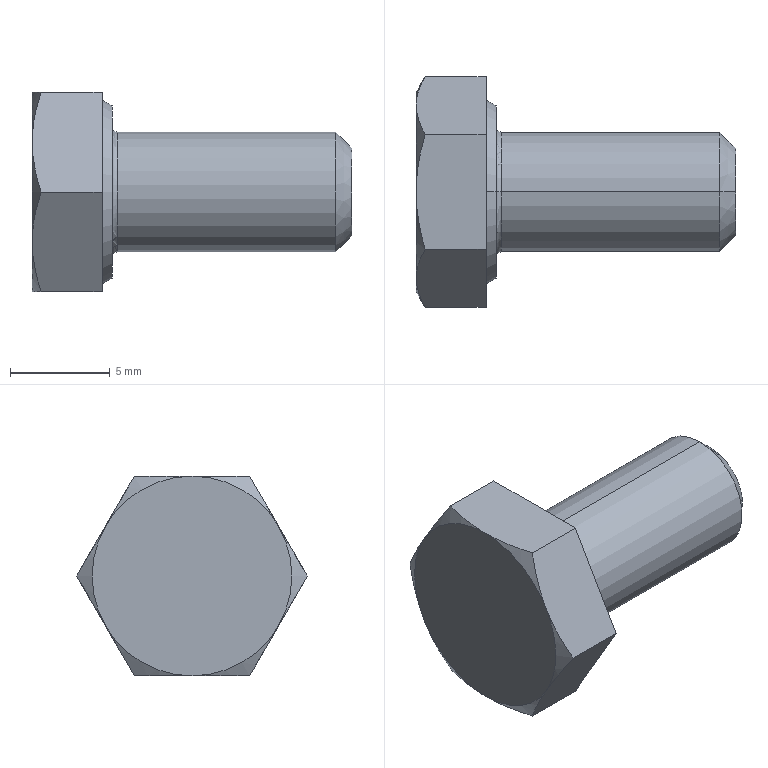Part | SolidWorks | features RevCut 3, Revolution 2, Chamfer 1, Extrusion 1 | 1 solid | 24 faces | box 16 x 11.547 x 10 mm | volume 667.282 mm3 | cone 10 | plane 10 | cylinder 2 | torus 2 | commonest cylinder face diameters 6 x2
STEP:
#1=CARTESIAN_POINT('',(4.25,0.,3.));
#2=VERTEX_POINT('',#1);
#3=CARTESIAN_POINT('',(4.25,0.,-3.));
#4=VERTEX_POINT('',#3);
#5=CARTESIAN_POINT('',(4.25,0.,0.));
#6=DIRECTION('',(-1.,0.,0.));
#7=DIRECTION('',(0.,0.,1.));
#8=AXIS2_PLACEMENT_3D('',#5,#6,#7);
#9=CIRCLE('',#8,3.);
#10=EDGE_CURVE('',#2,#4,#9,.T.);
#11=ORIENTED_EDGE('',*,*,#10,.F.);
#12=CARTESIAN_POINT('',(15.2,0.,3.));
#13=VERTEX_POINT('',#12);
#14=CARTESIAN_POINT('',(0.,0.,3.));
#15=DIRECTION('',(1.,0.,0.));
#16=VECTOR('',#15,1000.);
#17=LINE('',#14,#16);
#18=EDGE_CURVE('',#2,#13,#17,.T.);
#19=ORIENTED_EDGE('',*,*,#18,.T.);
#20=CARTESIAN_POINT('',(15.2,0.,-3.));
#21=VERTEX_POINT('',#20);
#22=CARTESIAN_POINT('',(15.2,0.,0.));
#23=DIRECTION('',(-1.,0.,0.));
#24=DIRECTION('',(0.,0.,-1.));
#25=AXIS2_PLACEMENT_3D('',#22,#23,#24);
#26=CIRCLE('',#25,3.);
#27=EDGE_CURVE('',#13,#21,#26,.T.);
#28=ORIENTED_EDGE('',*,*,#27,.T.);
#29=CARTESIAN_POINT('',(0.,0.,-3.));
#30=DIRECTION('',(1.,0.,0.));
#31=VECTOR('',#30,1000.);
#32=LINE('',#29,#31);
#33=EDGE_CURVE('',#4,#21,#32,.T.);
#34=ORIENTED_EDGE('',*,*,#33,.F.);
#35=EDGE_LOOP('',(#11,#19,#28,#34));
#36=FACE_OUTER_BOUND('',#35,.T.);
#37=CARTESIAN_POINT('',(0.,0.,0.));
#38=DIRECTION('',(1.,0.,0.));
#39=DIRECTION('',(0.,0.,-1.));
#40=AXIS2_PLACEMENT_3D('',#37,#38,#39);
#41=CYLINDRICAL_SURFACE('',#40,3.);
#42=ADVANCED_FACE('',(#36),#41,.T.);
#43=CARTESIAN_POINT('',(16.,0.,-2.2));
#44=VERTEX_POINT('',#43);
#45=CARTESIAN_POINT('',(16.,0.,2.2));
#46=VERTEX_POINT('',#45);
#47=CARTESIAN_POINT('',(16.,0.,0.));
#48=DIRECTION('',(1.,0.,0.));
#49=DIRECTION('',(0.,0.,-1.));
#50=AXIS2_PLACEMENT_3D('',#47,#48,#49);
#51=CIRCLE('',#50,2.2);
#52=EDGE_CURVE('',#44,#46,#51,.T.);
#53=ORIENTED_EDGE('',*,*,#52,.F.);
#54=CARTESIAN_POINT('',(16.,0.,-2.2));
#55=DIRECTION('',(-0.7071,0.,-0.7071));
#56=VECTOR('',#55,1000.);
#57=LINE('',#54,#56);
#58=EDGE_CURVE('',#44,#21,#57,.T.);
#59=ORIENTED_EDGE('',*,*,#58,.T.);
#60=ORIENTED_EDGE('',*,*,#27,.F.);
#61=CARTESIAN_POINT('',(16.,0.,2.2));
#62=DIRECTION('',(-0.7071,0.,0.7071));
#63=VECTOR('',#62,1000.);
#64=LINE('',#61,#63);
#65=EDGE_CURVE('',#46,#13,#64,.T.);
#66=ORIENTED_EDGE('',*,*,#65,.F.);
#67=EDGE_LOOP('',(#53,#59,#60,#66));
#68=FACE_OUTER_BOUND('',#67,.T.);
#69=CARTESIAN_POINT('',(16.,0.,0.));
#70=DIRECTION('',(-1.,0.,0.));
#71=DIRECTION('',(0.,0.,1.));
#72=AXIS2_PLACEMENT_3D('',#69,#70,#71);
#73=CONICAL_SURFACE('',#72,2.2,0.7854);
#74=ADVANCED_FACE('',(#68),#73,.T.);
#75=CARTESIAN_POINT('',(4.,0.,-3.25));
#76=VERTEX_POINT('',#75);
#77=CARTESIAN_POINT('',(4.,0.,3.25));
#78=VERTEX_POINT('',#77);
#79=CARTESIAN_POINT('',(4.,0.,0.));
#80=DIRECTION('',(-1.,0.,0.));
#81=DIRECTION('',(0.,0.,1.));
#82=AXIS2_PLACEMENT_3D('',#79,#80,#81);
#83=CIRCLE('',#82,3.25);
#84=EDGE_CURVE('',#76,#78,#83,.T.);
#85=ORIENTED_EDGE('',*,*,#84,.F.);
#86=CARTESIAN_POINT('',(4.25,0.,-3.25));
#87=DIRECTION('',(0.,1.,0.));
#88=DIRECTION('',(0.,0.,1.));
#89=AXIS2_PLACEMENT_3D('',#86,#87,#88);
#90=CIRCLE('',#89,0.25);
#91=EDGE_CURVE('',#76,#4,#90,.T.);
#92=ORIENTED_EDGE('',*,*,#91,.T.);
#93=CARTESIAN_POINT('',(4.25,0.,0.));
#94=DIRECTION('',(-1.,0.,0.));
#95=DIRECTION('',(0.,0.,1.));
#96=AXIS2_PLACEMENT_3D('',#93,#94,#95);
#97=CIRCLE('',#96,3.);
#98=EDGE_CURVE('',#4,#2,#97,.T.);
#99=ORIENTED_EDGE('',*,*,#98,.T.);
#100=CARTESIAN_POINT('',(4.25,0.,3.25));
#101=DIRECTION('',(0.,-1.,0.));
#102=DIRECTION('',(0.,0.,-1.));
#103=AXIS2_PLACEMENT_3D('',#100,#101,#102);
#104=CIRCLE('',#103,0.25);
#105=EDGE_CURVE('',#78,#2,#104,.T.);
#106=ORIENTED_EDGE('',*,*,#105,.F.);
#107=EDGE_LOOP('',(#85,#92,#99,#106));
#108=FACE_OUTER_BOUND('',#107,.T.);
#109=CARTESIAN_POINT('',(4.25,0.,0.));
#110=DIRECTION('',(-1.,0.,0.));
#111=DIRECTION('',(0.,0.,1.));
#112=AXIS2_PLACEMENT_3D('',#109,#110,#111);
#113=TOROIDAL_SURFACE('',#112,3.25,0.25);
#114=ADVANCED_FACE('',(#108),#113,.F.);
#115=CARTESIAN_POINT('',(4.,0.,4.312));
#116=VERTEX_POINT('',#115);
#117=CARTESIAN_POINT('',(4.,0.,-4.312));
#118=VERTEX_POINT('',#117);
#119=CARTESIAN_POINT('',(4.,0.,0.));
#120=DIRECTION('',(-1.,0.,0.));
#121=DIRECTION('',(0.,0.,1.));
#122=AXIS2_PLACEMENT_3D('',#119,#120,#121);
#123=CIRCLE('',#122,4.312);
#124=EDGE_CURVE('',#116,#118,#123,.T.);
#125=ORIENTED_EDGE('',*,*,#124,.T.);
#126=CARTESIAN_POINT('',(3.5,0.,-4.601));
#127=VERTEX_POINT('',#126);
#128=CARTESIAN_POINT('',(3.5,0.,-4.601));
#129=DIRECTION('',(-0.866,0.,-0.5));
#130=VECTOR('',#129,1000.);
#131=LINE('',#128,#130);
#132=EDGE_CURVE('',#118,#127,#131,.T.);
#133=ORIENTED_EDGE('',*,*,#132,.T.);
#134=CARTESIAN_POINT('',(3.5,0.,4.601));
#135=VERTEX_POINT('',#134);
#136=CARTESIAN_POINT('',(3.5,0.,0.));
#137=DIRECTION('',(-1.,0.,0.));
#138=DIRECTION('',(0.,0.,1.));
#139=AXIS2_PLACEMENT_3D('',#136,#137,#138);
#140=CIRCLE('',#139,4.601);
#141=EDGE_CURVE('',#135,#127,#140,.T.);
#142=ORIENTED_EDGE('',*,*,#141,.F.);
#143=CARTESIAN_POINT('',(3.5,0.,4.601));
#144=DIRECTION('',(-0.866,0.,0.5));
#145=VECTOR('',#144,1000.);
#146=LINE('',#143,#145);
#147=EDGE_CURVE('',#116,#135,#146,.T.);
#148=ORIENTED_EDGE('',*,*,#147,.F.);
#149=EDGE_LOOP('',(#125,#133,#142,#148));
#150=FACE_OUTER_BOUND('',#149,.T.);
#151=CARTESIAN_POINT('',(3.5,0.,0.));
#152=DIRECTION('',(-1.,0.,0.));
#153=DIRECTION('',(0.,0.,1.));
#154=AXIS2_PLACEMENT_3D('',#151,#152,#153);
#155=CONICAL_SURFACE('',#154,4.601,0.5236);
#156=ADVANCED_FACE('',(#150),#155,.T.);
#157=ORIENTED_EDGE('',*,*,#124,.F.);
#158=CARTESIAN_POINT('',(4.,0.,0.));
#159=DIRECTION('',(-1.,0.,0.));
#160=DIRECTION('',(0.,0.,1.));
#161=AXIS2_PLACEMENT_3D('',#158,#159,#160);
#162=CIRCLE('',#161,4.312);
#163=EDGE_CURVE('',#118,#116,#162,.T.);
#164=ORIENTED_EDGE('',*,*,#163,.F.);
#165=EDGE_LOOP('',(#157,#164));
#166=FACE_OUTER_BOUND('',#165,.T.);
#167=CARTESIAN_POINT('',(4.,0.,0.));
#168=DIRECTION('',(-1.,0.,0.));
#169=DIRECTION('',(0.,0.,1.));
#170=AXIS2_PLACEMENT_3D('',#167,#168,#169);
#171=CIRCLE('',#170,3.25);
#172=EDGE_CURVE('',#78,#76,#171,.T.);
#173=ORIENTED_EDGE('',*,*,#172,.T.);
#174=ORIENTED_EDGE('',*,*,#84,.T.);
#175=EDGE_LOOP('',(#173,#174));
#176=FACE_BOUND('',#175,.T.);
#177=CARTESIAN_POINT('',(4.,5.774,0.));
#178=DIRECTION('',(1.,0.,0.));
#179=DIRECTION('',(0.,0.,-1.));
#180=AXIS2_PLACEMENT_3D('',#177,#178,#179);
#181=PLANE('',#180);
#182=ADVANCED_FACE('',(#166,#176),#181,.T.);
#183=CARTESIAN_POINT('',(3.5,2.887,-5.));
#184=VERTEX_POINT('',#183);
#185=CARTESIAN_POINT('',(3.5,5.774,0.));
#186=VERTEX_POINT('',#185);
#187=CARTESIAN_POINT('',(3.5,2.887,-5.));
#188=DIRECTION('',(0.,0.5,0.866));
#189=VECTOR('',#188,1000.);
#190=LINE('',#187,#189);
#191=EDGE_CURVE('',#184,#186,#190,.T.);
#192=ORIENTED_EDGE('',*,*,#191,.F.);
#193=CARTESIAN_POINT('',(0.4466,2.887,-5.));
#194=VERTEX_POINT('',#193);
#195=CARTESIAN_POINT('',(4.,2.887,-5.));
#196=DIRECTION('',(-1.,0.,0.));
#197=VECTOR('',#196,1000.);
#198=LINE('',#195,#197);
#199=EDGE_CURVE('',#184,#194,#198,.T.);
#200=ORIENTED_EDGE('',*,*,#199,.T.);
#201=CARTESIAN_POINT('',(0.,4.33,-2.5));
#202=VERTEX_POINT('',#201);
#203=CARTESIAN_POINT('',(0.,4.33,-2.5));
#204=CARTESIAN_POINT('',(0.,4.208,-2.712));
#205=CARTESIAN_POINT('',(0.01056,4.085,-2.925));
#206=CARTESIAN_POINT('',(0.0514,3.841,-3.347));
#207=CARTESIAN_POINT('',(0.08166,3.72,-3.556));
#208=CARTESIAN_POINT('',(0.1983,3.36,-4.181));
#209=CARTESIAN_POINT('',(0.3106,3.122,-4.592));
#210=CARTESIAN_POINT('',(0.4466,2.887,-5.));
#211=B_SPLINE_CURVE_WITH_KNOTS('',3,(#203,#204,#205,#206,#207,#208,#209,#210),.UNSPECIFIED.,.F.,.F.,(4,2,2,4),(0.002921,0.003649,0.004376,0.005831),.UNSPECIFIED.);
#212=EDGE_CURVE('',#202,#194,#211,.T.);
#213=ORIENTED_EDGE('',*,*,#212,.F.);
#214=CARTESIAN_POINT('',(0.4466,5.774,0.));
#215=VERTEX_POINT('',#214);
#216=CARTESIAN_POINT('',(0.4466,5.774,0.));
#217=CARTESIAN_POINT('',(0.1739,5.301,-0.8179));
#218=CARTESIAN_POINT('',(0.,4.822,-1.648));
#219=CARTESIAN_POINT('',(0.,4.33,-2.5));
#220=B_SPLINE_CURVE_WITH_KNOTS('',3,(#216,#217,#218,#219),.UNSPECIFIED.,.F.,.F.,(4,4),(0.000000238,0.002921),.UNSPECIFIED.);
#221=EDGE_CURVE('',#215,#202,#220,.T.);
#222=ORIENTED_EDGE('',*,*,#221,.F.);
#223=CARTESIAN_POINT('',(4.,5.774,0.));
#224=DIRECTION('',(-1.,0.,0.));
#225=VECTOR('',#224,1000.);
#226=LINE('',#223,#225);
#227=EDGE_CURVE('',#186,#215,#226,.T.);
#228=ORIENTED_EDGE('',*,*,#227,.F.);
#229=EDGE_LOOP('',(#192,#200,#213,#222,#228));
#230=FACE_OUTER_BOUND('',#229,.T.);
#231=CARTESIAN_POINT('',(4.,2.887,-5.));
#232=DIRECTION('',(0.,-0.866,0.5));
#233=DIRECTION('',(0.,-0.5,-0.866));
#234=AXIS2_PLACEMENT_3D('',#231,#232,#233);
#235=PLANE('',#234);
#236=ADVANCED_FACE('',(#230),#235,.F.);
#237=CARTESIAN_POINT('',(3.5,2.887,5.));
#238=VERTEX_POINT('',#237);
#239=CARTESIAN_POINT('',(3.5,5.774,0.));
#240=DIRECTION('',(0.,-0.5,0.866));
#241=VECTOR('',#240,1000.);
#242=LINE('',#239,#241);
#243=EDGE_CURVE('',#186,#238,#242,.T.);
#244=ORIENTED_EDGE('',*,*,#243,.F.);
#245=ORIENTED_EDGE('',*,*,#227,.T.);
#246=CARTESIAN_POINT('',(0.,4.33,2.5));
#247=VERTEX_POINT('',#246);
#248=CARTESIAN_POINT('',(0.,4.33,2.5));
#249=CARTESIAN_POINT('',(0.,4.453,2.288));
#250=CARTESIAN_POINT('',(0.01056,4.576,2.075));
#251=CARTESIAN_POINT('',(0.0514,4.819,1.653));
#252=CARTESIAN_POINT('',(0.08166,4.94,1.444));
#253=CARTESIAN_POINT('',(0.1983,5.3,0.8193));
#254=CARTESIAN_POINT('',(0.3106,5.538,0.4079));
#255=CARTESIAN_POINT('',(0.4466,5.774,0.));
#256=B_SPLINE_CURVE_WITH_KNOTS('',3,(#248,#249,#250,#251,#252,#253,#254,#255),.UNSPECIFIED.,.F.,.F.,(4,2,2,4),(0.002921,0.003649,0.004376,0.005831),.UNSPECIFIED.);
#257=EDGE_CURVE('',#247,#215,#256,.T.);
#258=ORIENTED_EDGE('',*,*,#257,.F.);
#259=CARTESIAN_POINT('',(0.4466,2.887,5.));
#260=VERTEX_POINT('',#259);
#261=CARTESIAN_POINT('',(0.4466,2.887,5.));
#262=CARTESIAN_POINT('',(0.1739,3.359,4.182));
#263=CARTESIAN_POINT('',(0.,3.838,3.352));
#264=CARTESIAN_POINT('',(0.,4.33,2.5));
#265=B_SPLINE_CURVE_WITH_KNOTS('',3,(#261,#262,#263,#264),.UNSPECIFIED.,.F.,.F.,(4,4),(0.000000238,0.002921),.UNSPECIFIED.);
#266=EDGE_CURVE('',#260,#247,#265,.T.);
#267=ORIENTED_EDGE('',*,*,#266,.F.);
#268=CARTESIAN_POINT('',(4.,2.887,5.));
#269=DIRECTION('',(-1.,0.,0.));
#270=VECTOR('',#269,1000.);
#271=LINE('',#268,#270);
#272=EDGE_CURVE('',#238,#260,#271,.T.);
#273=ORIENTED_EDGE('',*,*,#272,.F.);
#274=EDGE_LOOP('',(#244,#245,#258,#267,#273));
#275=FACE_OUTER_BOUND('',#274,.T.);
#276=CARTESIAN_POINT('',(4.,5.774,0.));
#277=DIRECTION('',(0.,-0.866,-0.5));
#278=DIRECTION('',(0.,0.5,-0.866));
#279=AXIS2_PLACEMENT_3D('',#276,#277,#278);
#280=PLANE('',#279);
#281=ADVANCED_FACE('',(#275),#280,.F.);
#282=CARTESIAN_POINT('',(3.5,-2.887,5.));
#283=VERTEX_POINT('',#282);
#284=CARTESIAN_POINT('',(3.5,2.887,5.));
#285=DIRECTION('',(0.,-1.,0.));
#286=VECTOR('',#285,1000.);
#287=LINE('',#284,#286);
#288=EDGE_CURVE('',#238,#283,#287,.T.);
#289=ORIENTED_EDGE('',*,*,#288,.F.);
#290=ORIENTED_EDGE('',*,*,#272,.T.);
#291=CARTESIAN_POINT('',(0.,0.,5.));
#292=VERTEX_POINT('',#291);
#293=CARTESIAN_POINT('',(0.,0.,5.));
#294=CARTESIAN_POINT('',(0.,0.4887,5.));
#295=CARTESIAN_POINT('',(0.04321,0.9837,5.));
#296=CARTESIAN_POINT('',(0.1996,1.947,5.));
#297=CARTESIAN_POINT('',(0.3118,2.42,5.));
#298=CARTESIAN_POINT('',(0.4466,2.887,5.));
#299=B_SPLINE_CURVE_WITH_KNOTS('',3,(#293,#294,#295,#296,#297,#298),.UNSPECIFIED.,.F.,.F.,(4,2,4),(0.008262,0.009724,0.01119),.UNSPECIFIED.);
#300=EDGE_CURVE('',#292,#260,#299,.T.);
#301=ORIENTED_EDGE('',*,*,#300,.F.);
#302=CARTESIAN_POINT('',(0.4466,-2.887,5.));
#303=VERTEX_POINT('',#302);
#304=CARTESIAN_POINT('',(0.4466,-2.887,5.));
#305=CARTESIAN_POINT('',(0.3109,-2.417,5.));
#306=CARTESIAN_POINT('',(0.1973,-1.936,5.));
#307=CARTESIAN_POINT('',(0.04202,-0.9731,5.));
#308=CARTESIAN_POINT('',(0.,-0.4884,5.));
#309=CARTESIAN_POINT('',(0.,0.,5.));
#310=B_SPLINE_CURVE_WITH_KNOTS('',3,(#304,#305,#306,#307,#308,#309),.UNSPECIFIED.,.F.,.F.,(4,2,4),(0.00534,0.006801,0.008262),.UNSPECIFIED.);
#311=EDGE_CURVE('',#303,#292,#310,.T.);
#312=ORIENTED_EDGE('',*,*,#311,.F.);
#313=CARTESIAN_POINT('',(4.,-2.887,5.));
#314=DIRECTION('',(-1.,0.,0.));
#315=VECTOR('',#314,1000.);
#316=LINE('',#313,#315);
#317=EDGE_CURVE('',#283,#303,#316,.T.);
#318=ORIENTED_EDGE('',*,*,#317,.F.);
#319=EDGE_LOOP('',(#289,#290,#301,#312,#318));
#320=FACE_OUTER_BOUND('',#319,.T.);
#321=CARTESIAN_POINT('',(4.,2.887,5.));
#322=DIRECTION('',(0.,0.,-1.));
#323=DIRECTION('',(-1.,0.,0.));
#324=AXIS2_PLACEMENT_3D('',#321,#322,#323);
#325=PLANE('',#324);
#326=ADVANCED_FACE('',(#320),#325,.F.);
#327=CARTESIAN_POINT('',(3.5,-5.774,0.));
#328=VERTEX_POINT('',#327);
#329=CARTESIAN_POINT('',(3.5,-5.774,0.));
#330=DIRECTION('',(0.,-0.5,-0.866));
#331=VECTOR('',#330,1000.);
#332=LINE('',#329,#331);
#333=EDGE_CURVE('',#283,#328,#332,.T.);
#334=ORIENTED_EDGE('',*,*,#333,.F.);
#335=ORIENTED_EDGE('',*,*,#317,.T.);
#336=CARTESIAN_POINT('',(0.,-4.33,2.5));
#337=VERTEX_POINT('',#336);
#338=CARTESIAN_POINT('',(0.,-4.33,2.5));
#339=CARTESIAN_POINT('',(0.,-4.208,2.712));
#340=CARTESIAN_POINT('',(0.01056,-4.085,2.925));
#341=CARTESIAN_POINT('',(0.0514,-3.841,3.347));
#342=CARTESIAN_POINT('',(0.08166,-3.72,3.556));
#343=CARTESIAN_POINT('',(0.1983,-3.36,4.181));
#344=CARTESIAN_POINT('',(0.3106,-3.122,4.592));
#345=CARTESIAN_POINT('',(0.4466,-2.887,5.));
#346=B_SPLINE_CURVE_WITH_KNOTS('',3,(#338,#339,#340,#341,#342,#343,#344,#345),.UNSPECIFIED.,.F.,.F.,(4,2,2,4),(0.002921,0.003649,0.004376,0.005831),.UNSPECIFIED.);
#347=EDGE_CURVE('',#337,#303,#346,.T.);
#348=ORIENTED_EDGE('',*,*,#347,.F.);
#349=CARTESIAN_POINT('',(0.4466,-5.774,0.));
#350=VERTEX_POINT('',#349);
#351=CARTESIAN_POINT('',(0.4466,-5.774,0.));
#352=CARTESIAN_POINT('',(0.1739,-5.301,0.8179));
#353=CARTESIAN_POINT('',(0.,-4.822,1.648));
#354=CARTESIAN_POINT('',(0.,-4.33,2.5));
#355=B_SPLINE_CURVE_WITH_KNOTS('',3,(#351,#352,#353,#354),.UNSPECIFIED.,.F.,.F.,(4,4),(0.000000238,0.002921),.UNSPECIFIED.);
#356=EDGE_CURVE('',#350,#337,#355,.T.);
#357=ORIENTED_EDGE('',*,*,#356,.F.);
#358=CARTESIAN_POINT('',(4.,-5.774,0.));
#359=DIRECTION('',(-1.,0.,0.));
#360=VECTOR('',#359,1000.);
#361=LINE('',#358,#360);
#362=EDGE_CURVE('',#328,#350,#361,.T.);
#363=ORIENTED_EDGE('',*,*,#362,.F.);
#364=EDGE_LOOP('',(#334,#335,#348,#357,#363));
#365=FACE_OUTER_BOUND('',#364,.T.);
#366=CARTESIAN_POINT('',(4.,-5.774,0.));
#367=DIRECTION('',(0.,0.866,-0.5));
#368=DIRECTION('',(0.,0.5,0.866));
#369=AXIS2_PLACEMENT_3D('',#366,#367,#368);
#370=PLANE('',#369);
#371=ADVANCED_FACE('',(#365),#370,.F.);
#372=CARTESIAN_POINT('',(3.5,-2.887,-5.));
#373=VERTEX_POINT('',#372);
#374=CARTESIAN_POINT('',(3.5,-2.887,-5.));
#375=DIRECTION('',(0.,0.5,-0.866));
#376=VECTOR('',#375,1000.);
#377=LINE('',#374,#376);
#378=EDGE_CURVE('',#328,#373,#377,.T.);
#379=ORIENTED_EDGE('',*,*,#378,.F.);
#380=ORIENTED_EDGE('',*,*,#362,.T.);
#381=CARTESIAN_POINT('',(0.,-4.33,-2.5));
#382=VERTEX_POINT('',#381);
#383=CARTESIAN_POINT('',(0.,-4.33,-2.5));
#384=CARTESIAN_POINT('',(0.,-4.453,-2.288));
#385=CARTESIAN_POINT('',(0.01056,-4.576,-2.075));
#386=CARTESIAN_POINT('',(0.0514,-4.819,-1.653));
#387=CARTESIAN_POINT('',(0.08166,-4.94,-1.444));
#388=CARTESIAN_POINT('',(0.1983,-5.3,-0.8193));
#389=CARTESIAN_POINT('',(0.3106,-5.538,-0.4079));
#390=CARTESIAN_POINT('',(0.4466,-5.774,0.));
#391=B_SPLINE_CURVE_WITH_KNOTS('',3,(#383,#384,#385,#386,#387,#388,#389,#390),.UNSPECIFIED.,.F.,.F.,(4,2,2,4),(0.002921,0.003649,0.004376,0.005831),.UNSPECIFIED.);
#392=EDGE_CURVE('',#382,#350,#391,.T.);
#393=ORIENTED_EDGE('',*,*,#392,.F.);
#394=CARTESIAN_POINT('',(0.4466,-2.887,-5.));
#395=VERTEX_POINT('',#394);
#396=CARTESIAN_POINT('',(0.4466,-2.887,-5.));
#397=CARTESIAN_POINT('',(0.1739,-3.359,-4.182));
#398=CARTESIAN_POINT('',(0.,-3.838,-3.352));
#399=CARTESIAN_POINT('',(0.,-4.33,-2.5));
#400=B_SPLINE_CURVE_WITH_KNOTS('',3,(#396,#397,#398,#399),.UNSPECIFIED.,.F.,.F.,(4,4),(0.000000238,0.002921),.UNSPECIFIED.);
#401=EDGE_CURVE('',#395,#382,#400,.T.);
#402=ORIENTED_EDGE('',*,*,#401,.F.);
#403=CARTESIAN_POINT('',(4.,-2.887,-5.));
#404=DIRECTION('',(-1.,0.,0.));
#405=VECTOR('',#404,1000.);
#406=LINE('',#403,#405);
#407=EDGE_CURVE('',#373,#395,#406,.T.);
#408=ORIENTED_EDGE('',*,*,#407,.F.);
#409=EDGE_LOOP('',(#379,#380,#393,#402,#408));
#410=FACE_OUTER_BOUND('',#409,.T.);
#411=CARTESIAN_POINT('',(4.,-2.887,-5.));
#412=DIRECTION('',(0.,0.866,0.5));
#413=DIRECTION('',(0.,-0.5,0.866));
#414=AXIS2_PLACEMENT_3D('',#411,#412,#413);
#415=PLANE('',#414);
#416=ADVANCED_FACE('',(#410),#415,.F.);
#417=CARTESIAN_POINT('',(3.5,2.887,-5.));
#418=DIRECTION('',(0.,1.,0.));
#419=VECTOR('',#418,1000.);
#420=LINE('',#417,#419);
#421=EDGE_CURVE('',#373,#184,#420,.T.);
#422=ORIENTED_EDGE('',*,*,#421,.F.);
#423=ORIENTED_EDGE('',*,*,#407,.T.);
#424=CARTESIAN_POINT('',(0.,0.,-5.));
#425=VERTEX_POINT('',#424);
#426=CARTESIAN_POINT('',(0.,0.,-5.));
#427=CARTESIAN_POINT('',(0.,-0.4884,-5.));
#428=CARTESIAN_POINT('',(0.04202,-0.9731,-5.));
#429=CARTESIAN_POINT('',(0.1973,-1.936,-5.));
#430=CARTESIAN_POINT('',(0.3109,-2.417,-5.));
#431=CARTESIAN_POINT('',(0.4466,-2.887,-5.));
#432=B_SPLINE_CURVE_WITH_KNOTS('',3,(#426,#427,#428,#429,#430,#431),.UNSPECIFIED.,.F.,.F.,(4,2,4),(0.01799,0.01945,0.02091),.UNSPECIFIED.);
#433=EDGE_CURVE('',#425,#395,#432,.T.);
#434=ORIENTED_EDGE('',*,*,#433,.F.);
#435=CARTESIAN_POINT('',(0.4466,2.887,-5.));
#436=CARTESIAN_POINT('',(0.3118,2.42,-5.));
#437=CARTESIAN_POINT('',(0.1996,1.947,-5.));
#438=CARTESIAN_POINT('',(0.04321,0.9837,-5.));
#439=CARTESIAN_POINT('',(0.,0.4887,-5.));
#440=CARTESIAN_POINT('',(0.,0.,-5.));
#441=B_SPLINE_CURVE_WITH_KNOTS('',3,(#435,#436,#437,#438,#439,#440),.UNSPECIFIED.,.F.,.F.,(4,2,4),(0.01507,0.01653,0.01799),.UNSPECIFIED.);
#442=EDGE_CURVE('',#194,#425,#441,.T.);
#443=ORIENTED_EDGE('',*,*,#442,.F.);
#444=ORIENTED_EDGE('',*,*,#199,.F.);
#445=EDGE_LOOP('',(#422,#423,#434,#443,#444));
#446=FACE_OUTER_BOUND('',#445,.T.);
#447=CARTESIAN_POINT('',(4.,2.887,-5.));
#448=DIRECTION('',(0.,0.,1.));
#449=DIRECTION('',(0.,-1.,0.));
#450=AXIS2_PLACEMENT_3D('',#447,#448,#449);
#451=PLANE('',#450);
#452=ADVANCED_FACE('',(#446),#451,.F.);
#453=ORIENTED_EDGE('',*,*,#401,.T.);
#454=CARTESIAN_POINT('',(0.,0.,0.));
#455=DIRECTION('',(1.,0.,0.));
#456=DIRECTION('',(0.,0.,-1.));
#457=AXIS2_PLACEMENT_3D('',#454,#455,#456);
#458=CIRCLE('',#457,5.);
#459=EDGE_CURVE('',#382,#425,#458,.T.);
#460=ORIENTED_EDGE('',*,*,#459,.T.);
#461=ORIENTED_EDGE('',*,*,#433,.T.);
#462=EDGE_LOOP('',(#453,#460,#461));
#463=FACE_OUTER_BOUND('',#462,.T.);
#464=CARTESIAN_POINT('',(0.,0.,0.));
#465=DIRECTION('',(1.,0.,0.));
#466=DIRECTION('',(0.,0.,-1.));
#467=AXIS2_PLACEMENT_3D('',#464,#465,#466);
#468=CONICAL_SURFACE('',#467,5.,1.047);
#469=ADVANCED_FACE('',(#463),#468,.T.);
#470=ORIENTED_EDGE('',*,*,#356,.T.);
#471=CARTESIAN_POINT('',(0.,0.,0.));
#472=DIRECTION('',(1.,0.,0.));
#473=DIRECTION('',(0.,0.,-1.));
#474=AXIS2_PLACEMENT_3D('',#471,#472,#473);
#475=CIRCLE('',#474,5.);
#476=EDGE_CURVE('',#337,#382,#475,.T.);
#477=ORIENTED_EDGE('',*,*,#476,.T.);
#478=ORIENTED_EDGE('',*,*,#392,.T.);
#479=EDGE_LOOP('',(#470,#477,#478));
#480=FACE_OUTER_BOUND('',#479,.T.);
#481=CARTESIAN_POINT('',(0.,0.,0.));
#482=DIRECTION('',(1.,0.,0.));
#483=DIRECTION('',(0.,0.,-1.));
#484=AXIS2_PLACEMENT_3D('',#481,#482,#483);
#485=CONICAL_SURFACE('',#484,5.,1.047);
#486=ADVANCED_FACE('',(#480),#485,.T.);
#487=ORIENTED_EDGE('',*,*,#311,.T.);
#488=CARTESIAN_POINT('',(0.,0.,0.));
#489=DIRECTION('',(1.,0.,0.));
#490=DIRECTION('',(0.,0.,-1.));
#491=AXIS2_PLACEMENT_3D('',#488,#489,#490);
#492=CIRCLE('',#491,5.);
#493=EDGE_CURVE('',#292,#337,#492,.T.);
#494=ORIENTED_EDGE('',*,*,#493,.T.);
#495=ORIENTED_EDGE('',*,*,#347,.T.);
#496=EDGE_LOOP('',(#487,#494,#495));
#497=FACE_OUTER_BOUND('',#496,.T.);
#498=CARTESIAN_POINT('',(0.,0.,0.));
#499=DIRECTION('',(1.,0.,0.));
#500=DIRECTION('',(0.,0.,-1.));
#501=AXIS2_PLACEMENT_3D('',#498,#499,#500);
#502=CONICAL_SURFACE('',#501,5.,1.047);
#503=ADVANCED_FACE('',(#497),#502,.T.);
#504=ORIENTED_EDGE('',*,*,#300,.T.);
#505=ORIENTED_EDGE('',*,*,#266,.T.);
#506=CARTESIAN_POINT('',(0.,0.,0.));
#507=DIRECTION('',(-1.,0.,0.));
#508=DIRECTION('',(0.,0.,1.));
#509=AXIS2_PLACEMENT_3D('',#506,#507,#508);
#510=CIRCLE('',#509,5.);
#511=EDGE_CURVE('',#292,#247,#510,.T.);
#512=ORIENTED_EDGE('',*,*,#511,.F.);
#513=EDGE_LOOP('',(#504,#505,#512));
#514=FACE_OUTER_BOUND('',#513,.T.);
#515=CARTESIAN_POINT('',(0.,0.,0.));
#516=DIRECTION('',(1.,0.,0.));
#517=DIRECTION('',(0.,0.,-1.));
#518=AXIS2_PLACEMENT_3D('',#515,#516,#517);
#519=CONICAL_SURFACE('',#518,5.,1.047);
#520=ADVANCED_FACE('',(#514),#519,.T.);
#521=ORIENTED_EDGE('',*,*,#257,.T.);
#522=ORIENTED_EDGE('',*,*,#221,.T.);
#523=CARTESIAN_POINT('',(0.,0.,0.));
#524=DIRECTION('',(1.,0.,0.));
#525=DIRECTION('',(0.,0.,-1.));
#526=AXIS2_PLACEMENT_3D('',#523,#524,#525);
#527=CIRCLE('',#526,5.);
#528=EDGE_CURVE('',#202,#247,#527,.T.);
#529=ORIENTED_EDGE('',*,*,#528,.T.);
#530=EDGE_LOOP('',(#521,#522,#529));
#531=FACE_OUTER_BOUND('',#530,.T.);
#532=CARTESIAN_POINT('',(0.,0.,0.));
#533=DIRECTION('',(1.,0.,0.));
#534=DIRECTION('',(0.,0.,-1.));
#535=AXIS2_PLACEMENT_3D('',#532,#533,#534);
#536=CONICAL_SURFACE('',#535,5.,1.047);
#537=ADVANCED_FACE('',(#531),#536,.T.);
#538=ORIENTED_EDGE('',*,*,#212,.T.);
#539=ORIENTED_EDGE('',*,*,#442,.T.);
#540=CARTESIAN_POINT('',(0.,0.,0.));
#541=DIRECTION('',(1.,0.,0.));
#542=DIRECTION('',(0.,0.,-1.));
#543=AXIS2_PLACEMENT_3D('',#540,#541,#542);
#544=CIRCLE('',#543,5.);
#545=EDGE_CURVE('',#425,#202,#544,.T.);
#546=ORIENTED_EDGE('',*,*,#545,.T.);
#547=EDGE_LOOP('',(#538,#539,#546));
#548=FACE_OUTER_BOUND('',#547,.T.);
#549=CARTESIAN_POINT('',(0.,0.,0.));
#550=DIRECTION('',(1.,0.,0.));
#551=DIRECTION('',(0.,0.,-1.));
#552=AXIS2_PLACEMENT_3D('',#549,#550,#551);
#553=CONICAL_SURFACE('',#552,5.,1.047);
#554=ADVANCED_FACE('',(#548),#553,.T.);
#555=ORIENTED_EDGE('',*,*,#545,.F.);
#556=ORIENTED_EDGE('',*,*,#459,.F.);
#557=ORIENTED_EDGE('',*,*,#476,.F.);
#558=ORIENTED_EDGE('',*,*,#493,.F.);
#559=ORIENTED_EDGE('',*,*,#511,.T.);
#560=ORIENTED_EDGE('',*,*,#528,.F.);
#561=EDGE_LOOP('',(#555,#556,#557,#558,#559,#560));
#562=FACE_OUTER_BOUND('',#561,.T.);
#563=CARTESIAN_POINT('',(0.,5.774,0.));
#564=DIRECTION('',(1.,0.,0.));
#565=DIRECTION('',(0.,0.,-1.));
#566=AXIS2_PLACEMENT_3D('',#563,#564,#565);
#567=PLANE('',#566);
#568=ADVANCED_FACE('',(#562),#567,.F.);
#569=ORIENTED_EDGE('',*,*,#141,.T.);
#570=CARTESIAN_POINT('',(3.5,0.,0.));
#571=DIRECTION('',(-1.,0.,0.));
#572=DIRECTION('',(0.,0.,1.));
#573=AXIS2_PLACEMENT_3D('',#570,#571,#572);
#574=CIRCLE('',#573,4.601);
#575=EDGE_CURVE('',#127,#135,#574,.T.);
#576=ORIENTED_EDGE('',*,*,#575,.T.);
#577=EDGE_LOOP('',(#569,#576));
#578=FACE_BOUND('',#577,.T.);
#579=ORIENTED_EDGE('',*,*,#191,.T.);
#580=ORIENTED_EDGE('',*,*,#243,.T.);
#581=ORIENTED_EDGE('',*,*,#288,.T.);
#582=ORIENTED_EDGE('',*,*,#333,.T.);
#583=ORIENTED_EDGE('',*,*,#378,.T.);
#584=ORIENTED_EDGE('',*,*,#421,.T.);
#585=EDGE_LOOP('',(#579,#580,#581,#582,#583,#584));
#586=FACE_OUTER_BOUND('',#585,.T.);
#587=CARTESIAN_POINT('',(3.5,4.601,0.));
#588=DIRECTION('',(1.,0.,0.));
#589=DIRECTION('',(0.,0.,-1.));
#590=AXIS2_PLACEMENT_3D('',#587,#588,#589);
#591=PLANE('',#590);
#592=ADVANCED_FACE('',(#578,#586),#591,.T.);
#593=ORIENTED_EDGE('',*,*,#132,.F.);
#594=ORIENTED_EDGE('',*,*,#163,.T.);
#595=ORIENTED_EDGE('',*,*,#147,.T.);
#596=ORIENTED_EDGE('',*,*,#575,.F.);
#597=EDGE_LOOP('',(#593,#594,#595,#596));
#598=FACE_OUTER_BOUND('',#597,.T.);
#599=CARTESIAN_POINT('',(3.5,0.,0.));
#600=DIRECTION('',(-1.,0.,0.));
#601=DIRECTION('',(0.,0.,1.));
#602=AXIS2_PLACEMENT_3D('',#599,#600,#601);
#603=CONICAL_SURFACE('',#602,4.601,0.5236);
#604=ADVANCED_FACE('',(#598),#603,.T.);
#605=ORIENTED_EDGE('',*,*,#91,.F.);
#606=ORIENTED_EDGE('',*,*,#172,.F.);
#607=ORIENTED_EDGE('',*,*,#105,.T.);
#608=ORIENTED_EDGE('',*,*,#10,.T.);
#609=EDGE_LOOP('',(#605,#606,#607,#608));
#610=FACE_OUTER_BOUND('',#609,.T.);
#611=CARTESIAN_POINT('',(4.25,0.,0.));
#612=DIRECTION('',(-1.,0.,0.));
#613=DIRECTION('',(0.,0.,1.));
#614=AXIS2_PLACEMENT_3D('',#611,#612,#613);
#615=TOROIDAL_SURFACE('',#614,3.25,0.25);
#616=ADVANCED_FACE('',(#610),#615,.F.);
#617=CARTESIAN_POINT('',(16.,0.,0.));
#618=DIRECTION('',(1.,0.,0.));
#619=DIRECTION('',(0.,0.,-1.));
#620=AXIS2_PLACEMENT_3D('',#617,#618,#619);
#621=CIRCLE('',#620,2.2);
#622=EDGE_CURVE('',#46,#44,#621,.T.);
#623=ORIENTED_EDGE('',*,*,#622,.T.);
#624=ORIENTED_EDGE('',*,*,#52,.T.);
#625=EDGE_LOOP('',(#623,#624));
#626=FACE_OUTER_BOUND('',#625,.T.);
#627=CARTESIAN_POINT('',(16.,0.,0.));
#628=DIRECTION('',(1.,0.,0.));
#629=DIRECTION('',(0.,0.,-1.));
#630=AXIS2_PLACEMENT_3D('',#627,#628,#629);
#631=PLANE('',#630);
#632=ADVANCED_FACE('',(#626),#631,.T.);
#633=ORIENTED_EDGE('',*,*,#58,.F.);
#634=ORIENTED_EDGE('',*,*,#622,.F.);
#635=ORIENTED_EDGE('',*,*,#65,.T.);
#636=CARTESIAN_POINT('',(15.2,0.,0.));
#637=DIRECTION('',(-1.,0.,0.));
#638=DIRECTION('',(0.,0.,-1.));
#639=AXIS2_PLACEMENT_3D('',#636,#637,#638);
#640=CIRCLE('',#639,3.);
#641=EDGE_CURVE('',#21,#13,#640,.T.);
#642=ORIENTED_EDGE('',*,*,#641,.F.);
#643=EDGE_LOOP('',(#633,#634,#635,#642));
#644=FACE_OUTER_BOUND('',#643,.T.);
#645=CARTESIAN_POINT('',(16.,0.,0.));
#646=DIRECTION('',(-1.,0.,0.));
#647=DIRECTION('',(0.,0.,1.));
#648=AXIS2_PLACEMENT_3D('',#645,#646,#647);
#649=CONICAL_SURFACE('',#648,2.2,0.7854);
#650=ADVANCED_FACE('',(#644),#649,.T.);
#651=ORIENTED_EDGE('',*,*,#18,.F.);
#652=ORIENTED_EDGE('',*,*,#98,.F.);
#653=ORIENTED_EDGE('',*,*,#33,.T.);
#654=ORIENTED_EDGE('',*,*,#641,.T.);
#655=EDGE_LOOP('',(#651,#652,#653,#654));
#656=FACE_OUTER_BOUND('',#655,.T.);
#657=CARTESIAN_POINT('',(0.,0.,0.));
#658=DIRECTION('',(1.,0.,0.));
#659=DIRECTION('',(0.,0.,-1.));
#660=AXIS2_PLACEMENT_3D('',#657,#658,#659);
#661=CYLINDRICAL_SURFACE('',#660,3.);
#662=ADVANCED_FACE('',(#656),#661,.T.);
#663=CLOSED_SHELL('',(#42,#74,#114,#156,#182,#236,#281,#326,#371,#416,#452,#469,#486,#503,#520,#537,#554,#568,#592,#604,#616,#632,#650,#662));
#664=MANIFOLD_SOLID_BREP('',#663);
#665=CARTESIAN_POINT('',(0.,0.,0.));
#666=DIRECTION('',(0.,0.,1.));
#667=DIRECTION('',(1.,0.,0.));
#668=AXIS2_PLACEMENT_3D('',#665,#666,#667);
#669=(LENGTH_UNIT()NAMED_UNIT(*)SI_UNIT(.MILLI.,.METRE.));
#670=UNCERTAINTY_MEASURE_WITH_UNIT(LENGTH_MEASURE(0.00001),#669,'','');
#671=(NAMED_UNIT(*)PLANE_ANGLE_UNIT()SI_UNIT($,.RADIAN.));
#672=(NAMED_UNIT(*)SI_UNIT($,.STERADIAN.)SOLID_ANGLE_UNIT());
#673=(GEOMETRIC_REPRESENTATION_CONTEXT(3)GLOBAL_UNCERTAINTY_ASSIGNED_CONTEXT((#670))GLOBAL_UNIT_ASSIGNED_CONTEXT((#669,#671,#672))REPRESENTATION_CONTEXT('',''));
#674=ADVANCED_BREP_SHAPE_REPRESENTATION('',(#664,#668),#673);